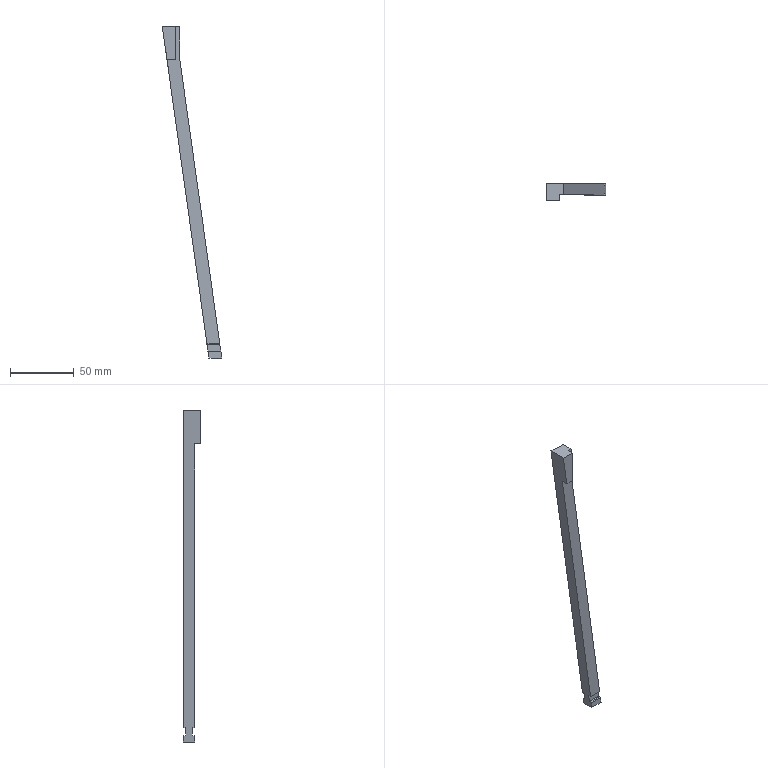Part | Creo | 1 solid | 23 faces | box 46.814 x 13.946 x 261.249 mm | volume 24943 mm3 | plane 19 | cylinder 4 | commonest cylinder face diameters 1 x4
STEP:
#1=CARTESIAN_POINT('',(-95.806,-121.035,38.749));
#2=VERTEX_POINT('',#1);
#3=CARTESIAN_POINT('',(-95.806,-134.875,38.749));
#4=VERTEX_POINT('',#3);
#5=CARTESIAN_POINT('',(-95.806,-121.035,38.749));
#6=DIRECTION('',(0.,-1.,0.));
#7=VECTOR('',#6,13.841);
#8=LINE('',#5,#7);
#9=EDGE_CURVE('',#2,#4,#8,.T.);
#10=ORIENTED_EDGE('',*,*,#9,.F.);
#11=CARTESIAN_POINT('',(-82.235,-121.035,38.231));
#12=VERTEX_POINT('',#11);
#13=CARTESIAN_POINT('',(-95.806,-121.035,38.749));
#14=DIRECTION('',(0.9993,0.,-0.03814));
#15=VECTOR('',#14,13.581);
#16=LINE('',#13,#15);
#17=EDGE_CURVE('',#2,#12,#16,.T.);
#18=ORIENTED_EDGE('',*,*,#17,.T.);
#19=CARTESIAN_POINT('',(-82.235,-129.93,38.231));
#20=VERTEX_POINT('',#19);
#21=CARTESIAN_POINT('',(-82.235,-129.93,38.231));
#22=DIRECTION('',(0.,1.,0.));
#23=VECTOR('',#22,8.895);
#24=LINE('',#21,#23);
#25=EDGE_CURVE('',#20,#12,#24,.T.);
#26=ORIENTED_EDGE('',*,*,#25,.F.);
#27=CARTESIAN_POINT('',(-85.454,-129.93,38.354));
#28=VERTEX_POINT('',#27);
#29=CARTESIAN_POINT('',(-82.235,-129.93,38.231));
#30=DIRECTION('',(-0.9993,0.,0.03814));
#31=VECTOR('',#30,3.221);
#32=LINE('',#29,#31);
#33=EDGE_CURVE('',#20,#28,#32,.T.);
#34=ORIENTED_EDGE('',*,*,#33,.T.);
#35=CARTESIAN_POINT('',(-85.454,-134.875,38.354));
#36=VERTEX_POINT('',#35);
#37=CARTESIAN_POINT('',(-85.454,-134.875,38.354));
#38=DIRECTION('',(0.,1.,0.));
#39=VECTOR('',#38,4.946);
#40=LINE('',#37,#39);
#41=EDGE_CURVE('',#36,#28,#40,.T.);
#42=ORIENTED_EDGE('',*,*,#41,.F.);
#43=CARTESIAN_POINT('',(-85.454,-134.875,38.354));
#44=DIRECTION('',(-0.9993,0.,0.03814));
#45=VECTOR('',#44,10.36);
#46=LINE('',#43,#45);
#47=EDGE_CURVE('',#36,#4,#46,.T.);
#48=ORIENTED_EDGE('',*,*,#47,.T.);
#49=EDGE_LOOP('',(#10,#18,#26,#34,#42,#48));
#50=FACE_OUTER_BOUND('',#49,.F.);
#51=CARTESIAN_POINT('',(-122.791,-167.242,39.779));
#52=DIRECTION('',(-0.03814,0.,-0.9993));
#53=DIRECTION('',(-0.9993,0.,0.03814));
#54=AXIS2_PLACEMENT_3D('',#51,#52,#53);
#55=PLANE('',#54);
#56=ADVANCED_FACE('',(#50),#55,.F.);
#57=CARTESIAN_POINT('',(-92.054,-129.93,12.054));
#58=VERTEX_POINT('',#57);
#59=CARTESIAN_POINT('',(-92.054,-134.875,12.054));
#60=VERTEX_POINT('',#59);
#61=CARTESIAN_POINT('',(-92.054,-129.93,12.054));
#62=DIRECTION('',(0.,-1.,0.));
#63=VECTOR('',#62,4.946);
#64=LINE('',#61,#63);
#65=EDGE_CURVE('',#58,#60,#64,.T.);
#66=ORIENTED_EDGE('',*,*,#65,.F.);
#67=CARTESIAN_POINT('',(-60.664,-129.93,-211.3));
#68=VERTEX_POINT('',#67);
#69=CARTESIAN_POINT('',(-92.054,-129.93,12.054));
#70=DIRECTION('',(0.1392,0.,-0.9903));
#71=VECTOR('',#70,225.549);
#72=LINE('',#69,#71);
#73=EDGE_CURVE('',#58,#68,#72,.T.);
#74=ORIENTED_EDGE('',*,*,#73,.T.);
#75=CARTESIAN_POINT('',(-60.664,-128.43,-211.3));
#76=VERTEX_POINT('',#75);
#77=CARTESIAN_POINT('',(-60.664,-129.93,-211.3));
#78=DIRECTION('',(0.,1.,0.));
#79=VECTOR('',#78,1.5);
#80=LINE('',#77,#79);
#81=EDGE_CURVE('',#68,#76,#80,.T.);
#82=ORIENTED_EDGE('',*,*,#81,.T.);
#83=CARTESIAN_POINT('',(-60.594,-127.93,-211.8));
#84=VERTEX_POINT('',#83);
#85=CARTESIAN_POINT('',(-60.664,-128.262,-211.3));
#86=CARTESIAN_POINT('',(-60.646,-128.055,-211.427));
#87=CARTESIAN_POINT('',(-60.617,-127.93,-211.634));
#88=CARTESIAN_POINT('',(-60.594,-127.93,-211.8));
#89=B_SPLINE_CURVE_WITH_KNOTS('',3,(#75,#85,#86,#87,#88),.UNSPECIFIED.,.F.,.F.,(4,1,4),(0.,0.5,1.),.UNSPECIFIED.);
#90=EDGE_CURVE('',#76,#84,#89,.T.);
#91=ORIENTED_EDGE('',*,*,#90,.T.);
#92=CARTESIAN_POINT('',(-59.863,-127.93,-217.));
#93=VERTEX_POINT('',#92);
#94=CARTESIAN_POINT('',(-60.594,-127.93,-211.8));
#95=DIRECTION('',(0.1392,0.,-0.9903));
#96=VECTOR('',#95,5.251);
#97=LINE('',#94,#96);
#98=EDGE_CURVE('',#84,#93,#97,.T.);
#99=ORIENTED_EDGE('',*,*,#98,.T.);
#100=CARTESIAN_POINT('',(-59.793,-128.43,-217.5));
#101=VERTEX_POINT('',#100);
#102=CARTESIAN_POINT('',(-59.84,-127.93,-217.166));
#103=CARTESIAN_POINT('',(-59.811,-128.055,-217.373));
#104=CARTESIAN_POINT('',(-59.793,-128.262,-217.5));
#105=CARTESIAN_POINT('',(-59.793,-128.43,-217.5));
#106=B_SPLINE_CURVE_WITH_KNOTS('',3,(#92,#102,#103,#104,#105),.UNSPECIFIED.,.F.,.F.,(4,1,4),(0.,0.5,1.),.UNSPECIFIED.);
#107=EDGE_CURVE('',#93,#101,#106,.T.);
#108=ORIENTED_EDGE('',*,*,#107,.T.);
#109=CARTESIAN_POINT('',(-59.793,-129.93,-217.5));
#110=VERTEX_POINT('',#109);
#111=CARTESIAN_POINT('',(-59.793,-129.93,-217.5));
#112=DIRECTION('',(0.,1.,0.));
#113=VECTOR('',#112,1.5);
#114=LINE('',#111,#113);
#115=EDGE_CURVE('',#110,#101,#114,.T.);
#116=ORIENTED_EDGE('',*,*,#115,.F.);
#117=CARTESIAN_POINT('',(-59.09,-129.93,-222.5));
#118=VERTEX_POINT('',#117);
#119=CARTESIAN_POINT('',(-59.793,-129.93,-217.5));
#120=DIRECTION('',(0.1392,0.,-0.9903));
#121=VECTOR('',#120,5.049);
#122=LINE('',#119,#121);
#123=EDGE_CURVE('',#110,#118,#122,.T.);
#124=ORIENTED_EDGE('',*,*,#123,.T.);
#125=CARTESIAN_POINT('',(-59.09,-120.93,-222.5));
#126=VERTEX_POINT('',#125);
#127=CARTESIAN_POINT('',(-59.09,-120.93,-222.5));
#128=DIRECTION('',(0.,-1.,0.));
#129=VECTOR('',#128,9.);
#130=LINE('',#127,#129);
#131=EDGE_CURVE('',#126,#118,#130,.T.);
#132=ORIENTED_EDGE('',*,*,#131,.F.);
#133=CARTESIAN_POINT('',(-59.793,-120.93,-217.5));
#134=VERTEX_POINT('',#133);
#135=CARTESIAN_POINT('',(-59.09,-120.93,-222.5));
#136=DIRECTION('',(-0.1392,0.,0.9903));
#137=VECTOR('',#136,5.049);
#138=LINE('',#135,#137);
#139=EDGE_CURVE('',#126,#134,#138,.T.);
#140=ORIENTED_EDGE('',*,*,#139,.T.);
#141=CARTESIAN_POINT('',(-59.793,-122.43,-217.5));
#142=VERTEX_POINT('',#141);
#143=CARTESIAN_POINT('',(-59.793,-122.43,-217.5));
#144=DIRECTION('',(0.,1.,0.));
#145=VECTOR('',#144,1.5);
#146=LINE('',#143,#145);
#147=EDGE_CURVE('',#142,#134,#146,.T.);
#148=ORIENTED_EDGE('',*,*,#147,.F.);
#149=CARTESIAN_POINT('',(-59.863,-122.93,-217.));
#150=VERTEX_POINT('',#149);
#151=CARTESIAN_POINT('',(-59.793,-122.597,-217.5));
#152=CARTESIAN_POINT('',(-59.811,-122.804,-217.373));
#153=CARTESIAN_POINT('',(-59.84,-122.93,-217.166));
#154=CARTESIAN_POINT('',(-59.863,-122.93,-217.));
#155=B_SPLINE_CURVE_WITH_KNOTS('',3,(#141,#151,#152,#153,#154),.UNSPECIFIED.,.F.,.F.,(4,1,4),(0.,0.5,1.),.UNSPECIFIED.);
#156=EDGE_CURVE('',#142,#150,#155,.T.);
#157=ORIENTED_EDGE('',*,*,#156,.T.);
#158=CARTESIAN_POINT('',(-60.594,-122.93,-211.8));
#159=VERTEX_POINT('',#158);
#160=CARTESIAN_POINT('',(-59.863,-122.93,-217.));
#161=DIRECTION('',(-0.1392,0.,0.9903));
#162=VECTOR('',#161,5.251);
#163=LINE('',#160,#162);
#164=EDGE_CURVE('',#150,#159,#163,.T.);
#165=ORIENTED_EDGE('',*,*,#164,.T.);
#166=CARTESIAN_POINT('',(-60.664,-122.43,-211.3));
#167=VERTEX_POINT('',#166);
#168=CARTESIAN_POINT('',(-60.617,-122.93,-211.634));
#169=CARTESIAN_POINT('',(-60.646,-122.804,-211.427));
#170=CARTESIAN_POINT('',(-60.664,-122.597,-211.3));
#171=CARTESIAN_POINT('',(-60.664,-122.43,-211.3));
#172=B_SPLINE_CURVE_WITH_KNOTS('',3,(#158,#168,#169,#170,#171),.UNSPECIFIED.,.F.,.F.,(4,1,4),(0.,0.5,1.),.UNSPECIFIED.);
#173=EDGE_CURVE('',#159,#167,#172,.T.);
#174=ORIENTED_EDGE('',*,*,#173,.T.);
#175=CARTESIAN_POINT('',(-60.664,-120.93,-211.3));
#176=VERTEX_POINT('',#175);
#177=CARTESIAN_POINT('',(-60.664,-122.43,-211.3));
#178=DIRECTION('',(0.,1.,0.));
#179=VECTOR('',#178,1.5);
#180=LINE('',#177,#179);
#181=EDGE_CURVE('',#167,#176,#180,.T.);
#182=ORIENTED_EDGE('',*,*,#181,.T.);
#183=CARTESIAN_POINT('',(-94.105,-120.93,26.648));
#184=VERTEX_POINT('',#183);
#185=CARTESIAN_POINT('',(-60.664,-120.93,-211.3));
#186=DIRECTION('',(-0.1392,0.,0.9903));
#187=VECTOR('',#186,240.286);
#188=LINE('',#185,#187);
#189=EDGE_CURVE('',#176,#184,#188,.T.);
#190=ORIENTED_EDGE('',*,*,#189,.T.);
#191=CARTESIAN_POINT('',(-95.806,-121.035,38.749));
#192=DIRECTION('',(0.1392,0.008595,-0.9902));
#193=VECTOR('',#192,12.22);
#194=LINE('',#191,#193);
#195=EDGE_CURVE('',#2,#184,#194,.T.);
#196=ORIENTED_EDGE('',*,*,#195,.F.);
#197=ORIENTED_EDGE('',*,*,#9,.T.);
#198=CARTESIAN_POINT('',(-95.806,-134.875,38.749));
#199=DIRECTION('',(0.1392,0.,-0.9903));
#200=VECTOR('',#199,26.957);
#201=LINE('',#198,#200);
#202=EDGE_CURVE('',#4,#60,#201,.T.);
#203=ORIENTED_EDGE('',*,*,#202,.T.);
#204=EDGE_LOOP('',(#66,#74,#82,#91,#99,#108,#116,#124,#132,#140,#148,#157,#165,#174,#182,#190,#196,#197,#203));
#205=FACE_OUTER_BOUND('',#204,.F.);
#206=CARTESIAN_POINT('',(-92.111,-131.403,12.458));
#207=DIRECTION('',(-0.9903,0.,-0.1392));
#208=DIRECTION('',(0.1392,0.,-0.9903));
#209=AXIS2_PLACEMENT_3D('',#206,#207,#208);
#210=PLANE('',#209);
#211=ADVANCED_FACE('',(#205),#210,.T.);
#212=CARTESIAN_POINT('',(-85.568,-134.875,12.054));
#213=VERTEX_POINT('',#212);
#214=CARTESIAN_POINT('',(-85.568,-129.93,12.054));
#215=VERTEX_POINT('',#214);
#216=CARTESIAN_POINT('',(-85.568,-134.875,12.054));
#217=DIRECTION('',(0.,1.,0.));
#218=VECTOR('',#217,4.946);
#219=LINE('',#216,#218);
#220=EDGE_CURVE('',#213,#215,#219,.T.);
#221=ORIENTED_EDGE('',*,*,#220,.T.);
#222=CARTESIAN_POINT('',(-85.568,-129.93,12.054));
#223=DIRECTION('',(-1.,0.,0.));
#224=VECTOR('',#223,6.486);
#225=LINE('',#222,#224);
#226=EDGE_CURVE('',#215,#58,#225,.T.);
#227=ORIENTED_EDGE('',*,*,#226,.T.);
#228=ORIENTED_EDGE('',*,*,#65,.T.);
#229=CARTESIAN_POINT('',(-92.054,-134.875,12.054));
#230=DIRECTION('',(1.,0.,0.));
#231=VECTOR('',#230,6.486);
#232=LINE('',#229,#231);
#233=EDGE_CURVE('',#60,#213,#232,.T.);
#234=ORIENTED_EDGE('',*,*,#233,.T.);
#235=EDGE_LOOP('',(#221,#227,#228,#234));
#236=FACE_OUTER_BOUND('',#235,.F.);
#237=CARTESIAN_POINT('',(-0.003698,-18.777,12.054));
#238=DIRECTION('',(0.,0.,-1.));
#239=DIRECTION('',(0.,-1.,0.));
#240=AXIS2_PLACEMENT_3D('',#237,#238,#239);
#241=PLANE('',#240);
#242=ADVANCED_FACE('',(#236),#241,.T.);
#243=CARTESIAN_POINT('',(-85.568,-134.875,12.054));
#244=DIRECTION('',(0.004363,0.,1.));
#245=VECTOR('',#244,26.3);
#246=LINE('',#243,#245);
#247=EDGE_CURVE('',#213,#36,#246,.T.);
#248=ORIENTED_EDGE('',*,*,#247,.T.);
#249=ORIENTED_EDGE('',*,*,#41,.T.);
#250=CARTESIAN_POINT('',(-85.454,-129.93,38.354));
#251=DIRECTION('',(-0.004363,0.,-1.));
#252=VECTOR('',#251,26.3);
#253=LINE('',#250,#252);
#254=EDGE_CURVE('',#28,#215,#253,.T.);
#255=ORIENTED_EDGE('',*,*,#254,.T.);
#256=ORIENTED_EDGE('',*,*,#220,.F.);
#257=EDGE_LOOP('',(#248,#249,#255,#256));
#258=FACE_OUTER_BOUND('',#257,.F.);
#259=CARTESIAN_POINT('',(-85.454,-134.875,38.354));
#260=DIRECTION('',(-1.,0.,0.004363));
#261=DIRECTION('',(0.004363,0.,1.));
#262=AXIS2_PLACEMENT_3D('',#259,#260,#261);
#263=PLANE('',#262);
#264=ADVANCED_FACE('',(#258),#263,.F.);
#265=ORIENTED_EDGE('',*,*,#47,.F.);
#266=ORIENTED_EDGE('',*,*,#247,.F.);
#267=ORIENTED_EDGE('',*,*,#233,.F.);
#268=ORIENTED_EDGE('',*,*,#202,.F.);
#269=EDGE_LOOP('',(#265,#266,#267,#268));
#270=FACE_OUTER_BOUND('',#269,.F.);
#271=CARTESIAN_POINT('',(-91.983,-134.875,12.054));
#272=DIRECTION('',(0.,1.,0.));
#273=DIRECTION('',(-1.,0.,0.));
#274=AXIS2_PLACEMENT_3D('',#271,#272,#273);
#275=PLANE('',#274);
#276=ADVANCED_FACE('',(#270),#275,.F.);
#277=ORIENTED_EDGE('',*,*,#254,.F.);
#278=ORIENTED_EDGE('',*,*,#33,.F.);
#279=CARTESIAN_POINT('',(-82.235,-129.93,14.037));
#280=VERTEX_POINT('',#279);
#281=CARTESIAN_POINT('',(-82.235,-129.93,14.037));
#282=DIRECTION('',(0.,0.,1.));
#283=VECTOR('',#282,24.194);
#284=LINE('',#281,#283);
#285=EDGE_CURVE('',#280,#20,#284,.T.);
#286=ORIENTED_EDGE('',*,*,#285,.F.);
#287=CARTESIAN_POINT('',(-50.566,-129.93,-211.3));
#288=VERTEX_POINT('',#287);
#289=CARTESIAN_POINT('',(-50.566,-129.93,-211.3));
#290=DIRECTION('',(-0.1392,0.,0.9903));
#291=VECTOR('',#290,227.552);
#292=LINE('',#289,#291);
#293=EDGE_CURVE('',#288,#280,#292,.T.);
#294=ORIENTED_EDGE('',*,*,#293,.F.);
#295=CARTESIAN_POINT('',(-60.664,-129.93,-211.3));
#296=DIRECTION('',(1.,0.,0.));
#297=VECTOR('',#296,10.098);
#298=LINE('',#295,#297);
#299=EDGE_CURVE('',#68,#288,#298,.T.);
#300=ORIENTED_EDGE('',*,*,#299,.F.);
#301=ORIENTED_EDGE('',*,*,#73,.F.);
#302=ORIENTED_EDGE('',*,*,#226,.F.);
#303=EDGE_LOOP('',(#277,#278,#286,#294,#300,#301,#302));
#304=FACE_OUTER_BOUND('',#303,.F.);
#305=CARTESIAN_POINT('',(-76.316,-129.93,199.798));
#306=DIRECTION('',(0.,1.,0.));
#307=DIRECTION('',(-1.,0.,0.));
#308=AXIS2_PLACEMENT_3D('',#305,#306,#307);
#309=PLANE('',#308);
#310=ADVANCED_FACE('',(#304),#309,.F.);
#311=CARTESIAN_POINT('',(-82.235,-120.93,26.195));
#312=VERTEX_POINT('',#311);
#313=CARTESIAN_POINT('',(-82.235,-120.93,14.037));
#314=VERTEX_POINT('',#313);
#315=CARTESIAN_POINT('',(-82.235,-120.93,26.195));
#316=DIRECTION('',(0.,0.,-1.));
#317=VECTOR('',#316,12.158);
#318=LINE('',#315,#317);
#319=EDGE_CURVE('',#312,#314,#318,.T.);
#320=ORIENTED_EDGE('',*,*,#319,.T.);
#321=CARTESIAN_POINT('',(-82.235,-120.93,14.037));
#322=DIRECTION('',(0.,-1.,0.));
#323=VECTOR('',#322,9.);
#324=LINE('',#321,#323);
#325=EDGE_CURVE('',#314,#280,#324,.T.);
#326=ORIENTED_EDGE('',*,*,#325,.T.);
#327=ORIENTED_EDGE('',*,*,#285,.T.);
#328=ORIENTED_EDGE('',*,*,#25,.T.);
#329=CARTESIAN_POINT('',(-82.235,-120.93,26.195));
#330=DIRECTION('',(0.,-0.008727,1.));
#331=VECTOR('',#330,12.037);
#332=LINE('',#329,#331);
#333=EDGE_CURVE('',#312,#12,#332,.T.);
#334=ORIENTED_EDGE('',*,*,#333,.F.);
#335=EDGE_LOOP('',(#320,#326,#327,#328,#334));
#336=FACE_OUTER_BOUND('',#335,.F.);
#337=CARTESIAN_POINT('',(-82.235,-187.507,11.557));
#338=DIRECTION('',(1.,0.,0.));
#339=DIRECTION('',(0.,0.,1.));
#340=AXIS2_PLACEMENT_3D('',#337,#338,#339);
#341=PLANE('',#340);
#342=ADVANCED_FACE('',(#336),#341,.T.);
#343=ORIENTED_EDGE('',*,*,#189,.F.);
#344=CARTESIAN_POINT('',(-50.566,-120.93,-211.3));
#345=VERTEX_POINT('',#344);
#346=CARTESIAN_POINT('',(-50.566,-120.93,-211.3));
#347=DIRECTION('',(-1.,0.,0.));
#348=VECTOR('',#347,10.098);
#349=LINE('',#346,#348);
#350=EDGE_CURVE('',#345,#176,#349,.T.);
#351=ORIENTED_EDGE('',*,*,#350,.F.);
#352=CARTESIAN_POINT('',(-82.235,-120.93,14.037));
#353=DIRECTION('',(0.1392,0.,-0.9903));
#354=VECTOR('',#353,227.552);
#355=LINE('',#352,#354);
#356=EDGE_CURVE('',#314,#345,#355,.T.);
#357=ORIENTED_EDGE('',*,*,#356,.F.);
#358=ORIENTED_EDGE('',*,*,#319,.F.);
#359=CARTESIAN_POINT('',(-94.105,-120.93,26.648));
#360=DIRECTION('',(0.9993,0.,-0.03814));
#361=VECTOR('',#360,11.879);
#362=LINE('',#359,#361);
#363=EDGE_CURVE('',#184,#312,#362,.T.);
#364=ORIENTED_EDGE('',*,*,#363,.F.);
#365=EDGE_LOOP('',(#343,#351,#357,#358,#364));
#366=FACE_OUTER_BOUND('',#365,.F.);
#367=CARTESIAN_POINT('',(-70.022,-120.93,-90.804));
#368=DIRECTION('',(0.,-1.,0.));
#369=DIRECTION('',(0.,0.,-1.));
#370=AXIS2_PLACEMENT_3D('',#367,#368,#369);
#371=PLANE('',#370);
#372=ADVANCED_FACE('',(#366),#371,.F.);
#373=CARTESIAN_POINT('',(-50.566,-122.43,-211.3));
#374=VERTEX_POINT('',#373);
#375=CARTESIAN_POINT('',(-50.566,-120.93,-211.3));
#376=DIRECTION('',(0.,-1.,0.));
#377=VECTOR('',#376,1.5);
#378=LINE('',#375,#377);
#379=EDGE_CURVE('',#345,#374,#378,.T.);
#380=ORIENTED_EDGE('',*,*,#379,.F.);
#381=ORIENTED_EDGE('',*,*,#350,.T.);
#382=ORIENTED_EDGE('',*,*,#181,.F.);
#383=CARTESIAN_POINT('',(-60.664,-122.43,-211.3));
#384=DIRECTION('',(1.,0.,0.));
#385=VECTOR('',#384,10.098);
#386=LINE('',#383,#385);
#387=EDGE_CURVE('',#167,#374,#386,.T.);
#388=ORIENTED_EDGE('',*,*,#387,.T.);
#389=EDGE_LOOP('',(#380,#381,#382,#388));
#390=FACE_OUTER_BOUND('',#389,.F.);
#391=CARTESIAN_POINT('',(64.001,21.659,-211.3));
#392=DIRECTION('',(0.,0.,-1.));
#393=DIRECTION('',(1.,0.,0.));
#394=AXIS2_PLACEMENT_3D('',#391,#392,#393);
#395=PLANE('',#394);
#396=ADVANCED_FACE('',(#390),#395,.T.);
#397=ORIENTED_EDGE('',*,*,#293,.T.);
#398=ORIENTED_EDGE('',*,*,#325,.F.);
#399=ORIENTED_EDGE('',*,*,#356,.T.);
#400=ORIENTED_EDGE('',*,*,#379,.T.);
#401=CARTESIAN_POINT('',(-50.496,-122.93,-211.8));
#402=VERTEX_POINT('',#401);
#403=CARTESIAN_POINT('',(-50.566,-122.43,-211.3));
#404=CARTESIAN_POINT('',(-50.566,-122.597,-211.3));
#405=CARTESIAN_POINT('',(-50.548,-122.804,-211.427));
#406=CARTESIAN_POINT('',(-50.519,-122.93,-211.634));
#407=CARTESIAN_POINT('',(-50.496,-122.93,-211.8));
#408=B_SPLINE_CURVE_WITH_KNOTS('',3,(#403,#404,#405,#406,#407),.UNSPECIFIED.,.F.,.F.,(4,1,4),(0.,0.5,1.),.UNSPECIFIED.);
#409=EDGE_CURVE('',#374,#402,#408,.T.);
#410=ORIENTED_EDGE('',*,*,#409,.T.);
#411=CARTESIAN_POINT('',(-49.765,-122.93,-217.));
#412=VERTEX_POINT('',#411);
#413=CARTESIAN_POINT('',(-50.496,-122.93,-211.8));
#414=DIRECTION('',(0.1392,0.,-0.9903));
#415=VECTOR('',#414,5.251);
#416=LINE('',#413,#415);
#417=EDGE_CURVE('',#402,#412,#416,.T.);
#418=ORIENTED_EDGE('',*,*,#417,.T.);
#419=CARTESIAN_POINT('',(-49.694,-122.43,-217.5));
#420=VERTEX_POINT('',#419);
#421=CARTESIAN_POINT('',(-49.765,-122.93,-217.));
#422=CARTESIAN_POINT('',(-49.741,-122.93,-217.166));
#423=CARTESIAN_POINT('',(-49.712,-122.804,-217.373));
#424=CARTESIAN_POINT('',(-49.694,-122.597,-217.5));
#425=CARTESIAN_POINT('',(-49.694,-122.43,-217.5));
#426=B_SPLINE_CURVE_WITH_KNOTS('',3,(#421,#422,#423,#424,#425),.UNSPECIFIED.,.F.,.F.,(4,1,4),(0.,0.5,1.),.UNSPECIFIED.);
#427=EDGE_CURVE('',#412,#420,#426,.T.);
#428=ORIENTED_EDGE('',*,*,#427,.T.);
#429=CARTESIAN_POINT('',(-49.694,-120.93,-217.5));
#430=VERTEX_POINT('',#429);
#431=CARTESIAN_POINT('',(-49.694,-120.93,-217.5));
#432=DIRECTION('',(0.,-1.,0.));
#433=VECTOR('',#432,1.5);
#434=LINE('',#431,#433);
#435=EDGE_CURVE('',#430,#420,#434,.T.);
#436=ORIENTED_EDGE('',*,*,#435,.F.);
#437=CARTESIAN_POINT('',(-48.992,-120.93,-222.5));
#438=VERTEX_POINT('',#437);
#439=CARTESIAN_POINT('',(-49.694,-120.93,-217.5));
#440=DIRECTION('',(0.1392,0.,-0.9903));
#441=VECTOR('',#440,5.049);
#442=LINE('',#439,#441);
#443=EDGE_CURVE('',#430,#438,#442,.T.);
#444=ORIENTED_EDGE('',*,*,#443,.T.);
#445=CARTESIAN_POINT('',(-48.992,-129.93,-222.5));
#446=VERTEX_POINT('',#445);
#447=CARTESIAN_POINT('',(-48.992,-129.93,-222.5));
#448=DIRECTION('',(0.,1.,0.));
#449=VECTOR('',#448,9.);
#450=LINE('',#447,#449);
#451=EDGE_CURVE('',#446,#438,#450,.T.);
#452=ORIENTED_EDGE('',*,*,#451,.F.);
#453=CARTESIAN_POINT('',(-49.694,-129.93,-217.5));
#454=VERTEX_POINT('',#453);
#455=CARTESIAN_POINT('',(-48.992,-129.93,-222.5));
#456=DIRECTION('',(-0.1392,0.,0.9903));
#457=VECTOR('',#456,5.049);
#458=LINE('',#455,#457);
#459=EDGE_CURVE('',#446,#454,#458,.T.);
#460=ORIENTED_EDGE('',*,*,#459,.T.);
#461=CARTESIAN_POINT('',(-49.694,-128.43,-217.5));
#462=VERTEX_POINT('',#461);
#463=CARTESIAN_POINT('',(-49.694,-128.43,-217.5));
#464=DIRECTION('',(0.,-1.,0.));
#465=VECTOR('',#464,1.5);
#466=LINE('',#463,#465);
#467=EDGE_CURVE('',#462,#454,#466,.T.);
#468=ORIENTED_EDGE('',*,*,#467,.F.);
#469=CARTESIAN_POINT('',(-49.765,-127.93,-217.));
#470=VERTEX_POINT('',#469);
#471=CARTESIAN_POINT('',(-49.694,-128.43,-217.5));
#472=CARTESIAN_POINT('',(-49.694,-128.262,-217.5));
#473=CARTESIAN_POINT('',(-49.712,-128.055,-217.373));
#474=CARTESIAN_POINT('',(-49.741,-127.93,-217.166));
#475=CARTESIAN_POINT('',(-49.765,-127.93,-217.));
#476=B_SPLINE_CURVE_WITH_KNOTS('',3,(#471,#472,#473,#474,#475),.UNSPECIFIED.,.F.,.F.,(4,1,4),(0.,0.5,1.),.UNSPECIFIED.);
#477=EDGE_CURVE('',#462,#470,#476,.T.);
#478=ORIENTED_EDGE('',*,*,#477,.T.);
#479=CARTESIAN_POINT('',(-50.496,-127.93,-211.8));
#480=VERTEX_POINT('',#479);
#481=CARTESIAN_POINT('',(-49.765,-127.93,-217.));
#482=DIRECTION('',(-0.1392,0.,0.9903));
#483=VECTOR('',#482,5.251);
#484=LINE('',#481,#483);
#485=EDGE_CURVE('',#470,#480,#484,.T.);
#486=ORIENTED_EDGE('',*,*,#485,.T.);
#487=CARTESIAN_POINT('',(-50.566,-128.43,-211.3));
#488=VERTEX_POINT('',#487);
#489=CARTESIAN_POINT('',(-50.496,-127.93,-211.8));
#490=CARTESIAN_POINT('',(-50.519,-127.93,-211.634));
#491=CARTESIAN_POINT('',(-50.548,-128.055,-211.427));
#492=CARTESIAN_POINT('',(-50.566,-128.262,-211.3));
#493=CARTESIAN_POINT('',(-50.566,-128.43,-211.3));
#494=B_SPLINE_CURVE_WITH_KNOTS('',3,(#489,#490,#491,#492,#493),.UNSPECIFIED.,.F.,.F.,(4,1,4),(0.,0.5,1.),.UNSPECIFIED.);
#495=EDGE_CURVE('',#480,#488,#494,.T.);
#496=ORIENTED_EDGE('',*,*,#495,.T.);
#497=CARTESIAN_POINT('',(-50.566,-128.43,-211.3));
#498=DIRECTION('',(0.,-1.,0.));
#499=VECTOR('',#498,1.5);
#500=LINE('',#497,#499);
#501=EDGE_CURVE('',#488,#288,#500,.T.);
#502=ORIENTED_EDGE('',*,*,#501,.T.);
#503=EDGE_LOOP('',(#397,#398,#399,#400,#410,#418,#428,#436,#444,#452,#460,#468,#478,#486,#496,#502));
#504=FACE_OUTER_BOUND('',#503,.F.);
#505=CARTESIAN_POINT('',(-82.209,-131.403,13.849));
#506=DIRECTION('',(-0.9903,0.,-0.1392));
#507=DIRECTION('',(0.1392,0.,-0.9903));
#508=AXIS2_PLACEMENT_3D('',#505,#506,#507);
#509=PLANE('',#508);
#510=ADVANCED_FACE('',(#504),#509,.F.);
#511=ORIENTED_EDGE('',*,*,#409,.F.);
#512=ORIENTED_EDGE('',*,*,#387,.F.);
#513=ORIENTED_EDGE('',*,*,#173,.F.);
#514=CARTESIAN_POINT('',(-50.496,-122.93,-211.8));
#515=DIRECTION('',(-1.,0.,0.));
#516=VECTOR('',#515,10.098);
#517=LINE('',#514,#516);
#518=EDGE_CURVE('',#402,#159,#517,.T.);
#519=ORIENTED_EDGE('',*,*,#518,.F.);
#520=EDGE_LOOP('',(#511,#512,#513,#519));
#521=FACE_OUTER_BOUND('',#520,.F.);
#522=CARTESIAN_POINT('',(64.001,-122.43,-211.8));
#523=DIRECTION('',(-1.,0.,0.));
#524=DIRECTION('',(0.,0.,1.));
#525=AXIS2_PLACEMENT_3D('',#522,#523,#524);
#526=CYLINDRICAL_SURFACE('',#525,0.5);
#527=ADVANCED_FACE('',(#521),#526,.F.);
#528=ORIENTED_EDGE('',*,*,#164,.F.);
#529=CARTESIAN_POINT('',(-59.863,-122.93,-217.));
#530=DIRECTION('',(1.,0.,0.));
#531=VECTOR('',#530,10.098);
#532=LINE('',#529,#531);
#533=EDGE_CURVE('',#150,#412,#532,.T.);
#534=ORIENTED_EDGE('',*,*,#533,.T.);
#535=ORIENTED_EDGE('',*,*,#417,.F.);
#536=ORIENTED_EDGE('',*,*,#518,.T.);
#537=EDGE_LOOP('',(#528,#534,#535,#536));
#538=FACE_OUTER_BOUND('',#537,.F.);
#539=CARTESIAN_POINT('',(-41.999,-122.93,-217.5));
#540=DIRECTION('',(0.,-1.,0.));
#541=DIRECTION('',(0.,0.,-1.));
#542=AXIS2_PLACEMENT_3D('',#539,#540,#541);
#543=PLANE('',#542);
#544=ADVANCED_FACE('',(#538),#543,.F.);
#545=ORIENTED_EDGE('',*,*,#427,.F.);
#546=ORIENTED_EDGE('',*,*,#533,.F.);
#547=ORIENTED_EDGE('',*,*,#156,.F.);
#548=CARTESIAN_POINT('',(-49.694,-122.43,-217.5));
#549=DIRECTION('',(-1.,0.,0.));
#550=VECTOR('',#549,10.098);
#551=LINE('',#548,#550);
#552=EDGE_CURVE('',#420,#142,#551,.T.);
#553=ORIENTED_EDGE('',*,*,#552,.F.);
#554=EDGE_LOOP('',(#545,#546,#547,#553));
#555=FACE_OUTER_BOUND('',#554,.F.);
#556=CARTESIAN_POINT('',(-41.999,-122.43,-217.));
#557=DIRECTION('',(1.,0.,0.));
#558=DIRECTION('',(0.,0.,-1.));
#559=AXIS2_PLACEMENT_3D('',#556,#557,#558);
#560=CYLINDRICAL_SURFACE('',#559,0.5);
#561=ADVANCED_FACE('',(#555),#560,.F.);
#562=ORIENTED_EDGE('',*,*,#147,.T.);
#563=CARTESIAN_POINT('',(-49.694,-120.93,-217.5));
#564=DIRECTION('',(-1.,0.,0.));
#565=VECTOR('',#564,10.098);
#566=LINE('',#563,#565);
#567=EDGE_CURVE('',#430,#134,#566,.T.);
#568=ORIENTED_EDGE('',*,*,#567,.F.);
#569=ORIENTED_EDGE('',*,*,#435,.T.);
#570=ORIENTED_EDGE('',*,*,#552,.T.);
#571=EDGE_LOOP('',(#562,#568,#569,#570));
#572=FACE_OUTER_BOUND('',#571,.F.);
#573=CARTESIAN_POINT('',(-41.999,-119.33,-217.5));
#574=DIRECTION('',(0.,0.,-1.));
#575=DIRECTION('',(0.,1.,0.));
#576=AXIS2_PLACEMENT_3D('',#573,#574,#575);
#577=PLANE('',#576);
#578=ADVANCED_FACE('',(#572),#577,.F.);
#579=ORIENTED_EDGE('',*,*,#443,.F.);
#580=ORIENTED_EDGE('',*,*,#567,.T.);
#581=ORIENTED_EDGE('',*,*,#139,.F.);
#582=CARTESIAN_POINT('',(-59.09,-120.93,-222.5));
#583=DIRECTION('',(1.,0.,0.));
#584=VECTOR('',#583,10.098);
#585=LINE('',#582,#584);
#586=EDGE_CURVE('',#126,#438,#585,.T.);
#587=ORIENTED_EDGE('',*,*,#586,.T.);
#588=EDGE_LOOP('',(#579,#580,#581,#587));
#589=FACE_OUTER_BOUND('',#588,.F.);
#590=CARTESIAN_POINT('',(-70.022,-120.93,-90.804));
#591=DIRECTION('',(0.,-1.,0.));
#592=DIRECTION('',(0.,0.,-1.));
#593=AXIS2_PLACEMENT_3D('',#590,#591,#592);
#594=PLANE('',#593);
#595=ADVANCED_FACE('',(#589),#594,.F.);
#596=ORIENTED_EDGE('',*,*,#131,.T.);
#597=CARTESIAN_POINT('',(-48.992,-129.93,-222.5));
#598=DIRECTION('',(-1.,0.,0.));
#599=VECTOR('',#598,10.098);
#600=LINE('',#597,#599);
#601=EDGE_CURVE('',#446,#118,#600,.T.);
#602=ORIENTED_EDGE('',*,*,#601,.F.);
#603=ORIENTED_EDGE('',*,*,#451,.T.);
#604=ORIENTED_EDGE('',*,*,#586,.F.);
#605=EDGE_LOOP('',(#596,#602,#603,#604));
#606=FACE_OUTER_BOUND('',#605,.F.);
#607=CARTESIAN_POINT('',(-429.496,101.277,-222.5));
#608=DIRECTION('',(0.,0.,-1.));
#609=DIRECTION('',(0.,1.,0.));
#610=AXIS2_PLACEMENT_3D('',#607,#608,#609);
#611=PLANE('',#610);
#612=ADVANCED_FACE('',(#606),#611,.T.);
#613=ORIENTED_EDGE('',*,*,#123,.F.);
#614=CARTESIAN_POINT('',(-59.793,-129.93,-217.5));
#615=DIRECTION('',(1.,0.,0.));
#616=VECTOR('',#615,10.098);
#617=LINE('',#614,#616);
#618=EDGE_CURVE('',#110,#454,#617,.T.);
#619=ORIENTED_EDGE('',*,*,#618,.T.);
#620=ORIENTED_EDGE('',*,*,#459,.F.);
#621=ORIENTED_EDGE('',*,*,#601,.T.);
#622=EDGE_LOOP('',(#613,#619,#620,#621));
#623=FACE_OUTER_BOUND('',#622,.F.);
#624=CARTESIAN_POINT('',(-76.316,-129.93,199.798));
#625=DIRECTION('',(0.,1.,0.));
#626=DIRECTION('',(-1.,0.,0.));
#627=AXIS2_PLACEMENT_3D('',#624,#625,#626);
#628=PLANE('',#627);
#629=ADVANCED_FACE('',(#623),#628,.F.);
#630=ORIENTED_EDGE('',*,*,#467,.T.);
#631=ORIENTED_EDGE('',*,*,#618,.F.);
#632=ORIENTED_EDGE('',*,*,#115,.T.);
#633=CARTESIAN_POINT('',(-59.793,-128.43,-217.5));
#634=DIRECTION('',(1.,0.,0.));
#635=VECTOR('',#634,10.098);
#636=LINE('',#633,#635);
#637=EDGE_CURVE('',#101,#462,#636,.T.);
#638=ORIENTED_EDGE('',*,*,#637,.T.);
#639=EDGE_LOOP('',(#630,#631,#632,#638));
#640=FACE_OUTER_BOUND('',#639,.F.);
#641=CARTESIAN_POINT('',(-41.999,-127.93,-217.5));
#642=DIRECTION('',(0.,0.,-1.));
#643=DIRECTION('',(0.,1.,0.));
#644=AXIS2_PLACEMENT_3D('',#641,#642,#643);
#645=PLANE('',#644);
#646=ADVANCED_FACE('',(#640),#645,.F.);
#647=ORIENTED_EDGE('',*,*,#477,.F.);
#648=ORIENTED_EDGE('',*,*,#637,.F.);
#649=ORIENTED_EDGE('',*,*,#107,.F.);
#650=CARTESIAN_POINT('',(-49.765,-127.93,-217.));
#651=DIRECTION('',(-1.,0.,0.));
#652=VECTOR('',#651,10.098);
#653=LINE('',#650,#652);
#654=EDGE_CURVE('',#470,#93,#653,.T.);
#655=ORIENTED_EDGE('',*,*,#654,.F.);
#656=EDGE_LOOP('',(#647,#648,#649,#655));
#657=FACE_OUTER_BOUND('',#656,.F.);
#658=CARTESIAN_POINT('',(-41.999,-128.43,-217.));
#659=DIRECTION('',(1.,0.,0.));
#660=DIRECTION('',(0.,0.,-1.));
#661=AXIS2_PLACEMENT_3D('',#658,#659,#660);
#662=CYLINDRICAL_SURFACE('',#661,0.5);
#663=ADVANCED_FACE('',(#657),#662,.F.);
#664=ORIENTED_EDGE('',*,*,#485,.F.);
#665=ORIENTED_EDGE('',*,*,#654,.T.);
#666=ORIENTED_EDGE('',*,*,#98,.F.);
#667=CARTESIAN_POINT('',(-60.594,-127.93,-211.8));
#668=DIRECTION('',(1.,0.,0.));
#669=VECTOR('',#668,10.098);
#670=LINE('',#667,#669);
#671=EDGE_CURVE('',#84,#480,#670,.T.);
#672=ORIENTED_EDGE('',*,*,#671,.T.);
#673=EDGE_LOOP('',(#664,#665,#666,#672));
#674=FACE_OUTER_BOUND('',#673,.F.);
#675=CARTESIAN_POINT('',(-41.999,-127.93,-212.3));
#676=DIRECTION('',(0.,1.,0.));
#677=DIRECTION('',(0.,0.,1.));
#678=AXIS2_PLACEMENT_3D('',#675,#676,#677);
#679=PLANE('',#678);
#680=ADVANCED_FACE('',(#674),#679,.F.);
#681=ORIENTED_EDGE('',*,*,#90,.F.);
#682=CARTESIAN_POINT('',(-50.566,-128.43,-211.3));
#683=DIRECTION('',(-1.,0.,0.));
#684=VECTOR('',#683,10.098);
#685=LINE('',#682,#684);
#686=EDGE_CURVE('',#488,#76,#685,.T.);
#687=ORIENTED_EDGE('',*,*,#686,.F.);
#688=ORIENTED_EDGE('',*,*,#495,.F.);
#689=ORIENTED_EDGE('',*,*,#671,.F.);
#690=EDGE_LOOP('',(#681,#687,#688,#689));
#691=FACE_OUTER_BOUND('',#690,.F.);
#692=CARTESIAN_POINT('',(64.001,-128.43,-211.8));
#693=DIRECTION('',(1.,0.,0.));
#694=DIRECTION('',(0.,0.,-1.));
#695=AXIS2_PLACEMENT_3D('',#692,#693,#694);
#696=CYLINDRICAL_SURFACE('',#695,0.5);
#697=ADVANCED_FACE('',(#691),#696,.F.);
#698=ORIENTED_EDGE('',*,*,#81,.F.);
#699=ORIENTED_EDGE('',*,*,#299,.T.);
#700=ORIENTED_EDGE('',*,*,#501,.F.);
#701=ORIENTED_EDGE('',*,*,#686,.T.);
#702=EDGE_LOOP('',(#698,#699,#700,#701));
#703=FACE_OUTER_BOUND('',#702,.F.);
#704=CARTESIAN_POINT('',(64.001,21.659,-211.3));
#705=DIRECTION('',(0.,0.,-1.));
#706=DIRECTION('',(1.,0.,0.));
#707=AXIS2_PLACEMENT_3D('',#704,#705,#706);
#708=PLANE('',#707);
#709=ADVANCED_FACE('',(#703),#708,.T.);
#710=ORIENTED_EDGE('',*,*,#333,.T.);
#711=ORIENTED_EDGE('',*,*,#17,.F.);
#712=ORIENTED_EDGE('',*,*,#195,.T.);
#713=ORIENTED_EDGE('',*,*,#363,.T.);
#714=EDGE_LOOP('',(#710,#711,#712,#713));
#715=FACE_OUTER_BOUND('',#714,.F.);
#716=CARTESIAN_POINT('',(-96.107,-121.035,38.76));
#717=DIRECTION('',(0.0003331,1.,0.008727));
#718=DIRECTION('',(0.,-0.008727,1.));
#719=AXIS2_PLACEMENT_3D('',#716,#717,#718);
#720=PLANE('',#719);
#721=ADVANCED_FACE('',(#715),#720,.T.);
#722=CLOSED_SHELL('',(#56,#211,#242,#264,#276,#310,#342,#372,#396,#510,#527,#544,#561,#578,#595,#612,#629,#646,#663,#680,#697,#709,#721));
#723=MANIFOLD_SOLID_BREP('',#722);
#724=(LENGTH_UNIT()NAMED_UNIT(*)SI_UNIT(.MILLI.,.METRE.));
#725=UNCERTAINTY_MEASURE_WITH_UNIT(LENGTH_MEASURE(0.02658),#724,'','');
#726=(NAMED_UNIT(*)PLANE_ANGLE_UNIT()SI_UNIT($,.RADIAN.));
#727=PLANE_ANGLE_MEASURE_WITH_UNIT(PLANE_ANGLE_MEASURE(0.01745),#726);
#728=(CONVERSION_BASED_UNIT('DEGREE',#727)NAMED_UNIT(*)PLANE_ANGLE_UNIT());
#729=(NAMED_UNIT(*)SI_UNIT($,.STERADIAN.)SOLID_ANGLE_UNIT());
#730=(GEOMETRIC_REPRESENTATION_CONTEXT(3)GLOBAL_UNCERTAINTY_ASSIGNED_CONTEXT((#725))GLOBAL_UNIT_ASSIGNED_CONTEXT((#724,#728,#729))REPRESENTATION_CONTEXT('',''));
#731=ADVANCED_BREP_SHAPE_REPRESENTATION('',(#723),#730);